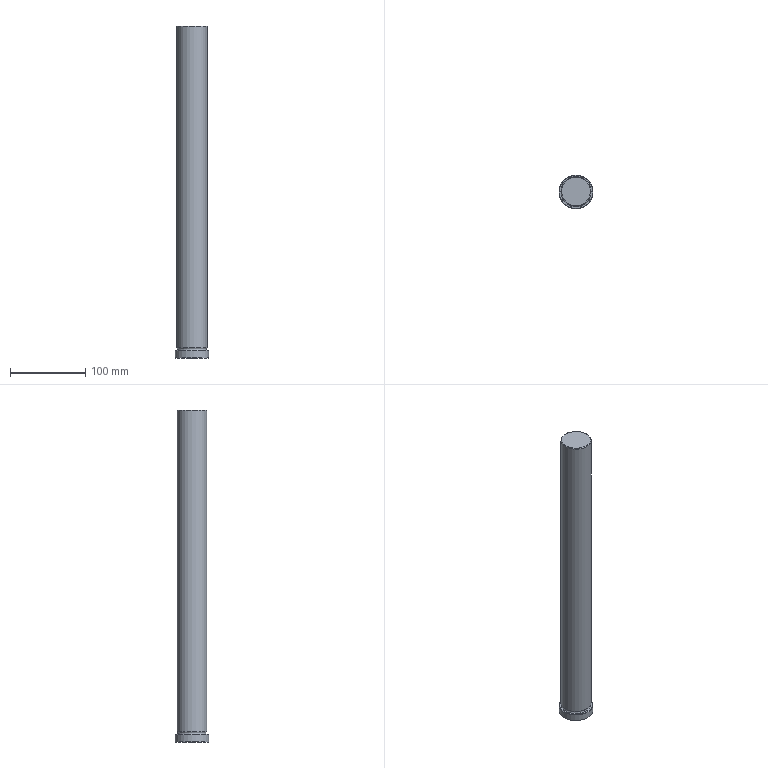Part | STEP file | solid 132 | 1 solid | 14 faces | box 45 x 45 x 440 mm | volume 555891 mm3 | plane 6 | cylinder 2 | torus 2 | cone 2 | other 1 | spline 1 | commonest cylinder face diameters 40 x1 45 x1